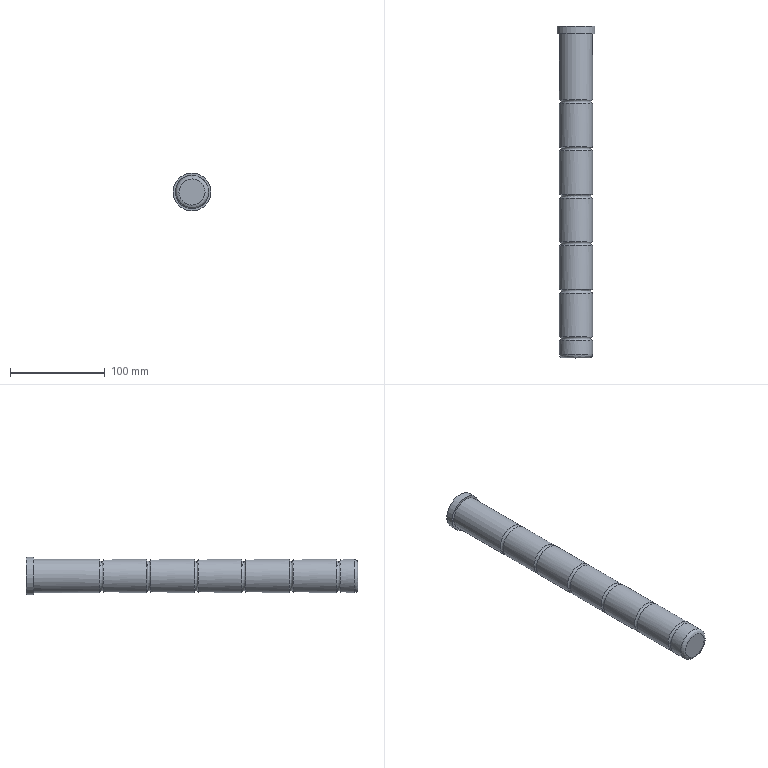Part | STEP file | GUIDE-PIN_id286_x_t | 1 solid | 18 faces | box 40 x 349.996 x 40 mm | volume 334779 mm3 | cylinder 8 | other 7 | plane 3 | commonest cylinder face diameters 35 x7 40 x1
STEP:
#1=CARTESIAN_POINT('',(148.25,-174.496,-160.));
#2=VERTEX_POINT('',#1);
#3=CARTESIAN_POINT('',(175.75,-174.496,-160.));
#4=VERTEX_POINT('',#3);
#5=CARTESIAN_POINT('',(148.25,-174.496,-160.));
#6=CARTESIAN_POINT('',(148.25,-174.496,-132.5));
#7=CARTESIAN_POINT('',(175.75,-174.496,-132.5));
#8=CARTESIAN_POINT('',(175.75,-174.496,-160.));
#9=(BOUNDED_CURVE()B_SPLINE_CURVE(3,(#5,#6,#7,#8),.UNSPECIFIED.,.F.,.F.)B_SPLINE_CURVE_WITH_KNOTS((4,4),(0.,1.),.UNSPECIFIED.)CURVE()GEOMETRIC_REPRESENTATION_ITEM()RATIONAL_B_SPLINE_CURVE((1.,0.3333,0.3333,1.))REPRESENTATION_ITEM(''));
#10=EDGE_CURVE('',#2,#4,#9,.T.);
#11=ORIENTED_EDGE('',*,*,#10,.F.);
#12=CARTESIAN_POINT('',(175.75,-174.496,-160.));
#13=CARTESIAN_POINT('',(175.75,-174.496,-187.5));
#14=CARTESIAN_POINT('',(148.25,-174.496,-187.5));
#15=CARTESIAN_POINT('',(148.25,-174.496,-160.));
#16=(BOUNDED_CURVE()B_SPLINE_CURVE(3,(#12,#13,#14,#15),.UNSPECIFIED.,.F.,.F.)B_SPLINE_CURVE_WITH_KNOTS((4,4),(0.,1.),.UNSPECIFIED.)CURVE()GEOMETRIC_REPRESENTATION_ITEM()RATIONAL_B_SPLINE_CURVE((1.,0.3333,0.3333,1.))REPRESENTATION_ITEM(''));
#17=EDGE_CURVE('',#4,#2,#16,.T.);
#18=ORIENTED_EDGE('',*,*,#17,.F.);
#19=EDGE_LOOP('',(#11,#18));
#20=FACE_OUTER_BOUND('',#19,.T.);
#21=CARTESIAN_POINT('',(162.,-174.496,-160.));
#22=DIRECTION('',(0.,1.,0.));
#23=DIRECTION('',(0.,0.,1.));
#24=AXIS2_PLACEMENT_3D('',#21,#22,#23);
#25=PLANE('',#24);
#26=ADVANCED_FACE('',(#20),#25,.F.);
#27=ORIENTED_EDGE('',*,*,#17,.T.);
#28=ORIENTED_EDGE('',*,*,#10,.T.);
#29=EDGE_LOOP('',(#27,#28));
#30=FACE_BOUND('',#29,.T.);
#31=CARTESIAN_POINT('',(162.,-170.746,-142.5));
#32=VERTEX_POINT('',#31);
#33=CARTESIAN_POINT('',(162.,-170.746,-160.));
#34=DIRECTION('',(0.,1.,0.));
#35=DIRECTION('',(0.,0.,1.));
#36=AXIS2_PLACEMENT_3D('',#33,#34,#35);
#37=CIRCLE('',#36,17.5);
#38=EDGE_CURVE('',#32,#32,#37,.T.);
#39=ORIENTED_EDGE('',*,*,#38,.F.);
#40=EDGE_LOOP('',(#39));
#41=FACE_BOUND('',#40,.T.);
#42=CARTESIAN_POINT('',(175.75,-170.746,-160.));
#43=DIRECTION('',(0.,0.,-1.));
#44=DIRECTION('',(1.,0.,0.));
#45=AXIS2_PLACEMENT_3D('',#42,#43,#44);
#46=CIRCLE('',#45,3.75);
#47=CARTESIAN_POINT('',(162.,-170.746,-160.));
#48=DIRECTION('',(0.,1.,0.));
#49=AXIS1_PLACEMENT('',#47,#48);
#50=SURFACE_OF_REVOLUTION('',#46,#49);
#51=ADVANCED_FACE('',(#30,#41),#50,.F.);
#52=ORIENTED_EDGE('',*,*,#38,.T.);
#53=EDGE_LOOP('',(#52));
#54=FACE_BOUND('',#53,.T.);
#55=CARTESIAN_POINT('',(179.5,-156.02,-160.));
#56=VERTEX_POINT('',#55);
#57=CARTESIAN_POINT('',(162.,-156.02,-160.));
#58=DIRECTION('',(0.,-1.,0.));
#59=DIRECTION('',(1.,0.,0.));
#60=AXIS2_PLACEMENT_3D('',#57,#58,#59);
#61=CIRCLE('',#60,17.5);
#62=EDGE_CURVE('',#56,#56,#61,.T.);
#63=ORIENTED_EDGE('',*,*,#62,.T.);
#64=EDGE_LOOP('',(#63));
#65=FACE_BOUND('',#64,.T.);
#66=CARTESIAN_POINT('',(162.,-191.996,-160.));
#67=DIRECTION('',(0.,1.,0.));
#68=DIRECTION('',(0.,0.,1.));
#69=AXIS2_PLACEMENT_3D('',#66,#67,#68);
#70=CYLINDRICAL_SURFACE('',#69,17.5);
#71=ADVANCED_FACE('',(#54,#65),#70,.T.);
#72=ORIENTED_EDGE('',*,*,#62,.F.);
#73=EDGE_LOOP('',(#72));
#74=FACE_BOUND('',#73,.T.);
#75=CARTESIAN_POINT('',(162.,-152.02,-142.5));
#76=VERTEX_POINT('',#75);
#77=CARTESIAN_POINT('',(162.,-152.02,-160.));
#78=DIRECTION('',(0.,1.,0.));
#79=DIRECTION('',(0.,0.,1.));
#80=AXIS2_PLACEMENT_3D('',#77,#78,#79);
#81=CIRCLE('',#80,17.5);
#82=EDGE_CURVE('',#76,#76,#81,.T.);
#83=ORIENTED_EDGE('',*,*,#82,.F.);
#84=EDGE_LOOP('',(#83));
#85=FACE_BOUND('',#84,.T.);
#86=CARTESIAN_POINT('',(179.48,-154.02,-160.));
#87=DIRECTION('',(0.,0.,-1.));
#88=DIRECTION('',(1.,0.,0.));
#89=AXIS2_PLACEMENT_3D('',#86,#87,#88);
#90=CIRCLE('',#89,2.);
#91=CARTESIAN_POINT('',(162.,-154.02,-160.));
#92=DIRECTION('',(0.,1.,0.));
#93=AXIS1_PLACEMENT('',#91,#92);
#94=SURFACE_OF_REVOLUTION('',#90,#93);
#95=ADVANCED_FACE('',(#74,#85),#94,.T.);
#96=ORIENTED_EDGE('',*,*,#82,.T.);
#97=EDGE_LOOP('',(#96));
#98=FACE_BOUND('',#97,.T.);
#99=CARTESIAN_POINT('',(179.5,-106.02,-160.));
#100=VERTEX_POINT('',#99);
#101=CARTESIAN_POINT('',(162.,-106.02,-160.));
#102=DIRECTION('',(0.,-1.,0.));
#103=DIRECTION('',(1.,0.,0.));
#104=AXIS2_PLACEMENT_3D('',#101,#102,#103);
#105=CIRCLE('',#104,17.5);
#106=EDGE_CURVE('',#100,#100,#105,.T.);
#107=ORIENTED_EDGE('',*,*,#106,.T.);
#108=EDGE_LOOP('',(#107));
#109=FACE_BOUND('',#108,.T.);
#110=CARTESIAN_POINT('',(162.,-191.996,-160.));
#111=DIRECTION('',(0.,1.,0.));
#112=DIRECTION('',(0.,0.,1.));
#113=AXIS2_PLACEMENT_3D('',#110,#111,#112);
#114=CYLINDRICAL_SURFACE('',#113,17.5);
#115=ADVANCED_FACE('',(#98,#109),#114,.T.);
#116=ORIENTED_EDGE('',*,*,#106,.F.);
#117=EDGE_LOOP('',(#116));
#118=FACE_BOUND('',#117,.T.);
#119=CARTESIAN_POINT('',(162.,-102.02,-142.5));
#120=VERTEX_POINT('',#119);
#121=CARTESIAN_POINT('',(162.,-102.02,-160.));
#122=DIRECTION('',(0.,1.,0.));
#123=DIRECTION('',(0.,0.,1.));
#124=AXIS2_PLACEMENT_3D('',#121,#122,#123);
#125=CIRCLE('',#124,17.5);
#126=EDGE_CURVE('',#120,#120,#125,.T.);
#127=ORIENTED_EDGE('',*,*,#126,.F.);
#128=EDGE_LOOP('',(#127));
#129=FACE_BOUND('',#128,.T.);
#130=CARTESIAN_POINT('',(179.48,-104.02,-160.));
#131=DIRECTION('',(0.,0.,-1.));
#132=DIRECTION('',(1.,0.,0.));
#133=AXIS2_PLACEMENT_3D('',#130,#131,#132);
#134=CIRCLE('',#133,2.);
#135=CARTESIAN_POINT('',(162.,-104.02,-160.));
#136=DIRECTION('',(0.,1.,0.));
#137=AXIS1_PLACEMENT('',#135,#136);
#138=SURFACE_OF_REVOLUTION('',#134,#137);
#139=ADVANCED_FACE('',(#118,#129),#138,.T.);
#140=ORIENTED_EDGE('',*,*,#126,.T.);
#141=EDGE_LOOP('',(#140));
#142=FACE_BOUND('',#141,.T.);
#143=CARTESIAN_POINT('',(179.5,-56.02,-160.));
#144=VERTEX_POINT('',#143);
#145=CARTESIAN_POINT('',(162.,-56.02,-160.));
#146=DIRECTION('',(0.,-1.,0.));
#147=DIRECTION('',(1.,0.,0.));
#148=AXIS2_PLACEMENT_3D('',#145,#146,#147);
#149=CIRCLE('',#148,17.5);
#150=EDGE_CURVE('',#144,#144,#149,.T.);
#151=ORIENTED_EDGE('',*,*,#150,.T.);
#152=EDGE_LOOP('',(#151));
#153=FACE_BOUND('',#152,.T.);
#154=CARTESIAN_POINT('',(162.,-191.996,-160.));
#155=DIRECTION('',(0.,1.,0.));
#156=DIRECTION('',(0.,0.,1.));
#157=AXIS2_PLACEMENT_3D('',#154,#155,#156);
#158=CYLINDRICAL_SURFACE('',#157,17.5);
#159=ADVANCED_FACE('',(#142,#153),#158,.T.);
#160=ORIENTED_EDGE('',*,*,#150,.F.);
#161=EDGE_LOOP('',(#160));
#162=FACE_BOUND('',#161,.T.);
#163=CARTESIAN_POINT('',(162.,-52.02,-142.5));
#164=VERTEX_POINT('',#163);
#165=CARTESIAN_POINT('',(162.,-52.02,-160.));
#166=DIRECTION('',(0.,1.,0.));
#167=DIRECTION('',(0.,0.,1.));
#168=AXIS2_PLACEMENT_3D('',#165,#166,#167);
#169=CIRCLE('',#168,17.5);
#170=EDGE_CURVE('',#164,#164,#169,.T.);
#171=ORIENTED_EDGE('',*,*,#170,.F.);
#172=EDGE_LOOP('',(#171));
#173=FACE_BOUND('',#172,.T.);
#174=CARTESIAN_POINT('',(179.48,-54.02,-160.));
#175=DIRECTION('',(0.,0.,-1.));
#176=DIRECTION('',(1.,0.,0.));
#177=AXIS2_PLACEMENT_3D('',#174,#175,#176);
#178=CIRCLE('',#177,2.);
#179=CARTESIAN_POINT('',(162.,-54.02,-160.));
#180=DIRECTION('',(0.,1.,0.));
#181=AXIS1_PLACEMENT('',#179,#180);
#182=SURFACE_OF_REVOLUTION('',#178,#181);
#183=ADVANCED_FACE('',(#162,#173),#182,.T.);
#184=ORIENTED_EDGE('',*,*,#170,.T.);
#185=EDGE_LOOP('',(#184));
#186=FACE_BOUND('',#185,.T.);
#187=CARTESIAN_POINT('',(179.5,-6.02,-160.));
#188=VERTEX_POINT('',#187);
#189=CARTESIAN_POINT('',(162.,-6.02,-160.));
#190=DIRECTION('',(0.,-1.,0.));
#191=DIRECTION('',(1.,0.,0.));
#192=AXIS2_PLACEMENT_3D('',#189,#190,#191);
#193=CIRCLE('',#192,17.5);
#194=EDGE_CURVE('',#188,#188,#193,.T.);
#195=ORIENTED_EDGE('',*,*,#194,.T.);
#196=EDGE_LOOP('',(#195));
#197=FACE_BOUND('',#196,.T.);
#198=CARTESIAN_POINT('',(162.,-191.996,-160.));
#199=DIRECTION('',(0.,1.,0.));
#200=DIRECTION('',(0.,0.,1.));
#201=AXIS2_PLACEMENT_3D('',#198,#199,#200);
#202=CYLINDRICAL_SURFACE('',#201,17.5);
#203=ADVANCED_FACE('',(#186,#197),#202,.T.);
#204=ORIENTED_EDGE('',*,*,#194,.F.);
#205=EDGE_LOOP('',(#204));
#206=FACE_BOUND('',#205,.T.);
#207=CARTESIAN_POINT('',(162.,-2.02,-142.5));
#208=VERTEX_POINT('',#207);
#209=CARTESIAN_POINT('',(162.,-2.02,-160.));
#210=DIRECTION('',(0.,1.,0.));
#211=DIRECTION('',(0.,0.,1.));
#212=AXIS2_PLACEMENT_3D('',#209,#210,#211);
#213=CIRCLE('',#212,17.5);
#214=EDGE_CURVE('',#208,#208,#213,.T.);
#215=ORIENTED_EDGE('',*,*,#214,.F.);
#216=EDGE_LOOP('',(#215));
#217=FACE_BOUND('',#216,.T.);
#218=CARTESIAN_POINT('',(179.48,-4.02,-160.));
#219=DIRECTION('',(0.,0.,-1.));
#220=DIRECTION('',(1.,0.,0.));
#221=AXIS2_PLACEMENT_3D('',#218,#219,#220);
#222=CIRCLE('',#221,2.);
#223=CARTESIAN_POINT('',(162.,-4.02,-160.));
#224=DIRECTION('',(0.,1.,0.));
#225=AXIS1_PLACEMENT('',#223,#224);
#226=SURFACE_OF_REVOLUTION('',#222,#225);
#227=ADVANCED_FACE('',(#206,#217),#226,.T.);
#228=ORIENTED_EDGE('',*,*,#214,.T.);
#229=EDGE_LOOP('',(#228));
#230=FACE_BOUND('',#229,.T.);
#231=CARTESIAN_POINT('',(179.5,43.98,-160.));
#232=VERTEX_POINT('',#231);
#233=CARTESIAN_POINT('',(162.,43.98,-160.));
#234=DIRECTION('',(0.,-1.,0.));
#235=DIRECTION('',(1.,0.,0.));
#236=AXIS2_PLACEMENT_3D('',#233,#234,#235);
#237=CIRCLE('',#236,17.5);
#238=EDGE_CURVE('',#232,#232,#237,.T.);
#239=ORIENTED_EDGE('',*,*,#238,.T.);
#240=EDGE_LOOP('',(#239));
#241=FACE_BOUND('',#240,.T.);
#242=CARTESIAN_POINT('',(162.,-191.996,-160.));
#243=DIRECTION('',(0.,1.,0.));
#244=DIRECTION('',(0.,0.,1.));
#245=AXIS2_PLACEMENT_3D('',#242,#243,#244);
#246=CYLINDRICAL_SURFACE('',#245,17.5);
#247=ADVANCED_FACE('',(#230,#241),#246,.T.);
#248=CARTESIAN_POINT('',(162.,175.5,-140.));
#249=VERTEX_POINT('',#248);
#250=CARTESIAN_POINT('',(162.,175.5,-160.));
#251=DIRECTION('',(0.,-1.,0.));
#252=DIRECTION('',(0.,0.,1.));
#253=AXIS2_PLACEMENT_3D('',#250,#251,#252);
#254=CIRCLE('',#253,20.);
#255=EDGE_CURVE('',#249,#249,#254,.T.);
#256=ORIENTED_EDGE('',*,*,#255,.F.);
#257=EDGE_LOOP('',(#256));
#258=FACE_OUTER_BOUND('',#257,.T.);
#259=CARTESIAN_POINT('',(162.,175.5,-160.));
#260=DIRECTION('',(0.,1.,0.));
#261=DIRECTION('',(0.,0.,1.));
#262=AXIS2_PLACEMENT_3D('',#259,#260,#261);
#263=PLANE('',#262);
#264=ADVANCED_FACE('',(#258),#263,.T.);
#265=ORIENTED_EDGE('',*,*,#238,.F.);
#266=EDGE_LOOP('',(#265));
#267=FACE_BOUND('',#266,.T.);
#268=CARTESIAN_POINT('',(162.,47.98,-142.5));
#269=VERTEX_POINT('',#268);
#270=CARTESIAN_POINT('',(162.,47.98,-160.));
#271=DIRECTION('',(0.,1.,0.));
#272=DIRECTION('',(0.,0.,1.));
#273=AXIS2_PLACEMENT_3D('',#270,#271,#272);
#274=CIRCLE('',#273,17.5);
#275=EDGE_CURVE('',#269,#269,#274,.T.);
#276=ORIENTED_EDGE('',*,*,#275,.F.);
#277=EDGE_LOOP('',(#276));
#278=FACE_BOUND('',#277,.T.);
#279=CARTESIAN_POINT('',(179.48,45.98,-160.));
#280=DIRECTION('',(0.,0.,-1.));
#281=DIRECTION('',(1.,0.,0.));
#282=AXIS2_PLACEMENT_3D('',#279,#280,#281);
#283=CIRCLE('',#282,2.);
#284=CARTESIAN_POINT('',(162.,45.98,-160.));
#285=DIRECTION('',(0.,1.,0.));
#286=AXIS1_PLACEMENT('',#284,#285);
#287=SURFACE_OF_REVOLUTION('',#283,#286);
#288=ADVANCED_FACE('',(#267,#278),#287,.T.);
#289=CARTESIAN_POINT('',(162.,167.5,-140.));
#290=VERTEX_POINT('',#289);
#291=CARTESIAN_POINT('',(162.,167.5,-160.));
#292=DIRECTION('',(0.,1.,0.));
#293=DIRECTION('',(0.,0.,1.));
#294=AXIS2_PLACEMENT_3D('',#291,#292,#293);
#295=CIRCLE('',#294,20.);
#296=EDGE_CURVE('',#290,#290,#295,.T.);
#297=ORIENTED_EDGE('',*,*,#296,.T.);
#298=EDGE_LOOP('',(#297));
#299=FACE_BOUND('',#298,.T.);
#300=ORIENTED_EDGE('',*,*,#255,.T.);
#301=EDGE_LOOP('',(#300));
#302=FACE_BOUND('',#301,.T.);
#303=CARTESIAN_POINT('',(162.,-191.996,-160.));
#304=DIRECTION('',(0.,1.,0.));
#305=DIRECTION('',(0.,0.,1.));
#306=AXIS2_PLACEMENT_3D('',#303,#304,#305);
#307=CYLINDRICAL_SURFACE('',#306,20.);
#308=ADVANCED_FACE('',(#299,#302),#307,.T.);
#309=ORIENTED_EDGE('',*,*,#275,.T.);
#310=EDGE_LOOP('',(#309));
#311=FACE_BOUND('',#310,.T.);
#312=CARTESIAN_POINT('',(179.5,93.98,-160.));
#313=VERTEX_POINT('',#312);
#314=CARTESIAN_POINT('',(162.,93.98,-160.));
#315=DIRECTION('',(0.,-1.,0.));
#316=DIRECTION('',(1.,0.,0.));
#317=AXIS2_PLACEMENT_3D('',#314,#315,#316);
#318=CIRCLE('',#317,17.5);
#319=EDGE_CURVE('',#313,#313,#318,.T.);
#320=ORIENTED_EDGE('',*,*,#319,.T.);
#321=EDGE_LOOP('',(#320));
#322=FACE_BOUND('',#321,.T.);
#323=CARTESIAN_POINT('',(162.,-191.996,-160.));
#324=DIRECTION('',(0.,1.,0.));
#325=DIRECTION('',(0.,0.,1.));
#326=AXIS2_PLACEMENT_3D('',#323,#324,#325);
#327=CYLINDRICAL_SURFACE('',#326,17.5);
#328=ADVANCED_FACE('',(#311,#322),#327,.T.);
#329=CARTESIAN_POINT('',(162.,167.5,-142.5));
#330=VERTEX_POINT('',#329);
#331=CARTESIAN_POINT('',(162.,167.5,-160.));
#332=DIRECTION('',(0.,-1.,0.));
#333=DIRECTION('',(0.,0.,1.));
#334=AXIS2_PLACEMENT_3D('',#331,#332,#333);
#335=CIRCLE('',#334,17.5);
#336=EDGE_CURVE('',#330,#330,#335,.T.);
#337=ORIENTED_EDGE('',*,*,#336,.F.);
#338=EDGE_LOOP('',(#337));
#339=FACE_BOUND('',#338,.T.);
#340=ORIENTED_EDGE('',*,*,#296,.F.);
#341=EDGE_LOOP('',(#340));
#342=FACE_BOUND('',#341,.T.);
#343=CARTESIAN_POINT('',(162.,167.5,-160.));
#344=DIRECTION('',(0.,1.,0.));
#345=DIRECTION('',(0.,0.,1.));
#346=AXIS2_PLACEMENT_3D('',#343,#344,#345);
#347=PLANE('',#346);
#348=ADVANCED_FACE('',(#339,#342),#347,.F.);
#349=ORIENTED_EDGE('',*,*,#319,.F.);
#350=EDGE_LOOP('',(#349));
#351=FACE_BOUND('',#350,.T.);
#352=CARTESIAN_POINT('',(162.,97.98,-142.5));
#353=VERTEX_POINT('',#352);
#354=CARTESIAN_POINT('',(162.,97.98,-160.));
#355=DIRECTION('',(0.,1.,0.));
#356=DIRECTION('',(0.,0.,1.));
#357=AXIS2_PLACEMENT_3D('',#354,#355,#356);
#358=CIRCLE('',#357,17.5);
#359=EDGE_CURVE('',#353,#353,#358,.T.);
#360=ORIENTED_EDGE('',*,*,#359,.F.);
#361=EDGE_LOOP('',(#360));
#362=FACE_BOUND('',#361,.T.);
#363=CARTESIAN_POINT('',(179.48,95.98,-160.));
#364=DIRECTION('',(0.,0.,-1.));
#365=DIRECTION('',(1.,0.,0.));
#366=AXIS2_PLACEMENT_3D('',#363,#364,#365);
#367=CIRCLE('',#366,2.);
#368=CARTESIAN_POINT('',(162.,95.98,-160.));
#369=DIRECTION('',(0.,1.,0.));
#370=AXIS1_PLACEMENT('',#368,#369);
#371=SURFACE_OF_REVOLUTION('',#367,#370);
#372=ADVANCED_FACE('',(#351,#362),#371,.T.);
#373=ORIENTED_EDGE('',*,*,#359,.T.);
#374=EDGE_LOOP('',(#373));
#375=FACE_BOUND('',#374,.T.);
#376=ORIENTED_EDGE('',*,*,#336,.T.);
#377=EDGE_LOOP('',(#376));
#378=FACE_BOUND('',#377,.T.);
#379=CARTESIAN_POINT('',(162.,-191.996,-160.));
#380=DIRECTION('',(0.,1.,0.));
#381=DIRECTION('',(0.,0.,1.));
#382=AXIS2_PLACEMENT_3D('',#379,#380,#381);
#383=CYLINDRICAL_SURFACE('',#382,17.5);
#384=ADVANCED_FACE('',(#375,#378),#383,.T.);
#385=CLOSED_SHELL('',(#26,#51,#71,#95,#115,#139,#159,#183,#203,#227,#247,#264,#288,#308,#328,#348,#372,#384));
#386=MANIFOLD_SOLID_BREP('',#385);
#387=(LENGTH_UNIT()NAMED_UNIT(*)SI_UNIT(.MILLI.,.METRE.));
#388=UNCERTAINTY_MEASURE_WITH_UNIT(LENGTH_MEASURE(0.0508),#387,'','');
#389=(NAMED_UNIT(*)PLANE_ANGLE_UNIT()SI_UNIT($,.RADIAN.));
#390=PLANE_ANGLE_MEASURE_WITH_UNIT(PLANE_ANGLE_MEASURE(0.01745),#389);
#391=DIMENSIONAL_EXPONENTS(0.,0.,0.,0.,0.,0.,0.);
#392=(CONVERSION_BASED_UNIT('DEGREE',#390)NAMED_UNIT(#391)PLANE_ANGLE_UNIT());
#393=(NAMED_UNIT(*)SI_UNIT($,.STERADIAN.)SOLID_ANGLE_UNIT());
#394=(GEOMETRIC_REPRESENTATION_CONTEXT(3)GLOBAL_UNCERTAINTY_ASSIGNED_CONTEXT((#388))GLOBAL_UNIT_ASSIGNED_CONTEXT((#387,#392,#393))REPRESENTATION_CONTEXT('',''));
#395=ADVANCED_BREP_SHAPE_REPRESENTATION('',(#386),#394);